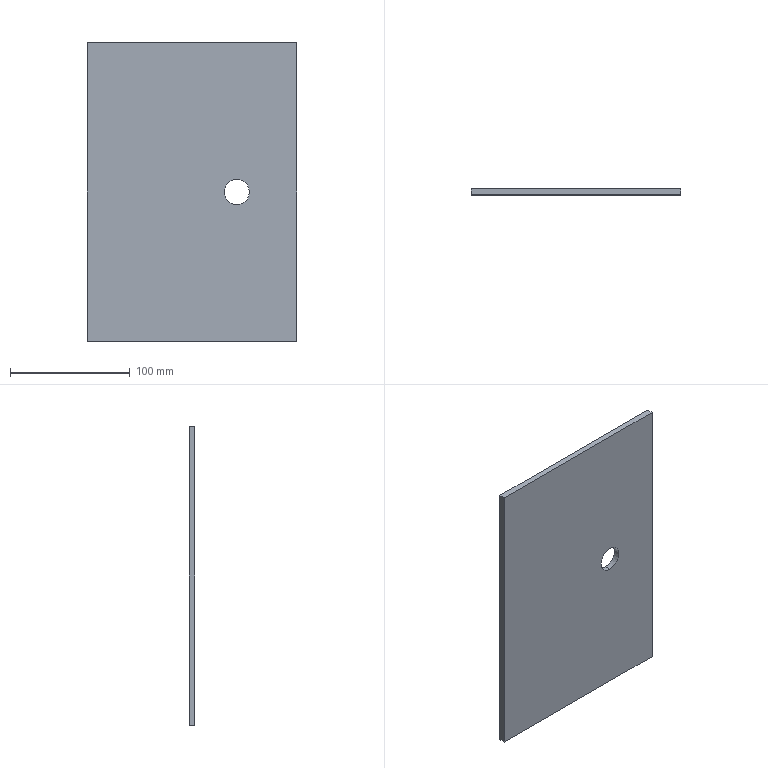Part | STEP file | Guide wheel mechanism revised.sldasm-Part-357 | 1 solid | 11 faces | box 175 x 5 x 250 mm | volume 216933 mm3 | plane 7 | cylinder 4 | commonest cylinder face diameters 6 x2 21 x2
STEP:
#1=CARTESIAN_POINT('',(0.,2.,54.));
#2=VERTEX_POINT('',#1);
#3=CARTESIAN_POINT('',(0.,2.,60.));
#4=VERTEX_POINT('',#3);
#5=CARTESIAN_POINT('',(0.,2.,57.));
#6=DIRECTION('',(0.,1.,0.));
#7=DIRECTION('',(0.,0.,1.));
#8=AXIS2_PLACEMENT_3D('',#5,#6,#7);
#9=CIRCLE('',#8,3.);
#10=EDGE_CURVE('',#2,#4,#9,.T.);
#11=ORIENTED_EDGE('',*,*,#10,.F.);
#12=CARTESIAN_POINT('',(0.,5.,54.));
#13=VERTEX_POINT('',#12);
#14=CARTESIAN_POINT('',(0.,2.,54.));
#15=DIRECTION('',(0.,1.,0.));
#16=VECTOR('',#15,1000.);
#17=LINE('',#14,#16);
#18=EDGE_CURVE('',#2,#13,#17,.T.);
#19=ORIENTED_EDGE('',*,*,#18,.T.);
#20=CARTESIAN_POINT('',(0.,5.,60.));
#21=VERTEX_POINT('',#20);
#22=CARTESIAN_POINT('',(0.,5.,57.));
#23=DIRECTION('',(0.,1.,0.));
#24=DIRECTION('',(0.,0.,1.));
#25=AXIS2_PLACEMENT_3D('',#22,#23,#24);
#26=CIRCLE('',#25,3.);
#27=EDGE_CURVE('',#13,#21,#26,.T.);
#28=ORIENTED_EDGE('',*,*,#27,.T.);
#29=CARTESIAN_POINT('',(0.,2.,60.));
#30=DIRECTION('',(0.,1.,0.));
#31=VECTOR('',#30,1000.);
#32=LINE('',#29,#31);
#33=EDGE_CURVE('',#4,#21,#32,.T.);
#34=ORIENTED_EDGE('',*,*,#33,.F.);
#35=EDGE_LOOP('',(#11,#19,#28,#34));
#36=FACE_OUTER_BOUND('',#35,.T.);
#37=CARTESIAN_POINT('',(0.,2.,57.));
#38=DIRECTION('',(0.,1.,0.));
#39=DIRECTION('',(0.,0.,1.));
#40=AXIS2_PLACEMENT_3D('',#37,#38,#39);
#41=CYLINDRICAL_SURFACE('',#40,3.);
#42=ADVANCED_FACE('',(#36),#41,.F.);
#43=CARTESIAN_POINT('',(0.,5.,-10.5));
#44=VERTEX_POINT('',#43);
#45=CARTESIAN_POINT('',(0.,5.,10.5));
#46=VERTEX_POINT('',#45);
#47=CARTESIAN_POINT('',(0.,5.,0.));
#48=DIRECTION('',(0.,1.,0.));
#49=DIRECTION('',(0.,0.,1.));
#50=AXIS2_PLACEMENT_3D('',#47,#48,#49);
#51=CIRCLE('',#50,10.5);
#52=EDGE_CURVE('',#44,#46,#51,.T.);
#53=ORIENTED_EDGE('',*,*,#52,.T.);
#54=CARTESIAN_POINT('',(0.,0.,10.5));
#55=VERTEX_POINT('',#54);
#56=CARTESIAN_POINT('',(0.,5.,10.5));
#57=DIRECTION('',(0.,-1.,0.));
#58=VECTOR('',#57,1000.);
#59=LINE('',#56,#58);
#60=EDGE_CURVE('',#46,#55,#59,.T.);
#61=ORIENTED_EDGE('',*,*,#60,.T.);
#62=CARTESIAN_POINT('',(0.,0.,-10.5));
#63=VERTEX_POINT('',#62);
#64=CARTESIAN_POINT('',(0.,0.,0.));
#65=DIRECTION('',(0.,1.,0.));
#66=DIRECTION('',(0.,0.,1.));
#67=AXIS2_PLACEMENT_3D('',#64,#65,#66);
#68=CIRCLE('',#67,10.5);
#69=EDGE_CURVE('',#63,#55,#68,.T.);
#70=ORIENTED_EDGE('',*,*,#69,.F.);
#71=CARTESIAN_POINT('',(0.,5.,-10.5));
#72=DIRECTION('',(0.,-1.,0.));
#73=VECTOR('',#72,1000.);
#74=LINE('',#71,#73);
#75=EDGE_CURVE('',#44,#63,#74,.T.);
#76=ORIENTED_EDGE('',*,*,#75,.F.);
#77=EDGE_LOOP('',(#53,#61,#70,#76));
#78=FACE_OUTER_BOUND('',#77,.T.);
#79=CARTESIAN_POINT('',(0.,5.,0.));
#80=DIRECTION('',(0.,-1.,0.));
#81=DIRECTION('',(0.,0.,-1.));
#82=AXIS2_PLACEMENT_3D('',#79,#80,#81);
#83=CYLINDRICAL_SURFACE('',#82,10.5);
#84=ADVANCED_FACE('',(#78),#83,.F.);
#85=CARTESIAN_POINT('',(50.,5.,-125.));
#86=VERTEX_POINT('',#85);
#87=CARTESIAN_POINT('',(50.,5.,125.));
#88=VERTEX_POINT('',#87);
#89=CARTESIAN_POINT('',(50.,5.,-125.));
#90=DIRECTION('',(0.,0.,1.));
#91=VECTOR('',#90,1000.);
#92=LINE('',#89,#91);
#93=EDGE_CURVE('',#86,#88,#92,.T.);
#94=ORIENTED_EDGE('',*,*,#93,.F.);
#95=CARTESIAN_POINT('',(-125.,5.,-125.));
#96=VERTEX_POINT('',#95);
#97=CARTESIAN_POINT('',(125.,5.,-125.));
#98=DIRECTION('',(-1.,0.,0.));
#99=VECTOR('',#98,1000.);
#100=LINE('',#97,#99);
#101=EDGE_CURVE('',#86,#96,#100,.T.);
#102=ORIENTED_EDGE('',*,*,#101,.T.);
#103=CARTESIAN_POINT('',(-125.,5.,125.));
#104=VERTEX_POINT('',#103);
#105=CARTESIAN_POINT('',(-125.,5.,125.));
#106=DIRECTION('',(0.,0.,1.));
#107=VECTOR('',#106,1000.);
#108=LINE('',#105,#107);
#109=EDGE_CURVE('',#96,#104,#108,.T.);
#110=ORIENTED_EDGE('',*,*,#109,.T.);
#111=CARTESIAN_POINT('',(125.,5.,125.));
#112=DIRECTION('',(1.,0.,0.));
#113=VECTOR('',#112,1000.);
#114=LINE('',#111,#113);
#115=EDGE_CURVE('',#104,#88,#114,.T.);
#116=ORIENTED_EDGE('',*,*,#115,.T.);
#117=EDGE_LOOP('',(#94,#102,#110,#116));
#118=FACE_OUTER_BOUND('',#117,.T.);
#119=CARTESIAN_POINT('',(0.,5.,57.));
#120=DIRECTION('',(0.,1.,0.));
#121=DIRECTION('',(0.,0.,1.));
#122=AXIS2_PLACEMENT_3D('',#119,#120,#121);
#123=CIRCLE('',#122,3.);
#124=EDGE_CURVE('',#21,#13,#123,.T.);
#125=ORIENTED_EDGE('',*,*,#124,.F.);
#126=ORIENTED_EDGE('',*,*,#27,.F.);
#127=EDGE_LOOP('',(#125,#126));
#128=FACE_BOUND('',#127,.T.);
#129=ORIENTED_EDGE('',*,*,#52,.F.);
#130=CARTESIAN_POINT('',(0.,5.,0.));
#131=DIRECTION('',(0.,1.,0.));
#132=DIRECTION('',(0.,0.,1.));
#133=AXIS2_PLACEMENT_3D('',#130,#131,#132);
#134=CIRCLE('',#133,10.5);
#135=EDGE_CURVE('',#46,#44,#134,.T.);
#136=ORIENTED_EDGE('',*,*,#135,.F.);
#137=EDGE_LOOP('',(#129,#136));
#138=FACE_BOUND('',#137,.T.);
#139=CARTESIAN_POINT('',(0.,5.,0.));
#140=DIRECTION('',(0.,1.,0.));
#141=DIRECTION('',(0.,0.,1.));
#142=AXIS2_PLACEMENT_3D('',#139,#140,#141);
#143=PLANE('',#142);
#144=ADVANCED_FACE('',(#118,#128,#138),#143,.T.);
#145=CARTESIAN_POINT('',(50.,0.,-125.));
#146=VERTEX_POINT('',#145);
#147=CARTESIAN_POINT('',(-125.,0.,-125.));
#148=VERTEX_POINT('',#147);
#149=CARTESIAN_POINT('',(125.,0.,-125.));
#150=DIRECTION('',(-1.,0.,0.));
#151=VECTOR('',#150,1000.);
#152=LINE('',#149,#151);
#153=EDGE_CURVE('',#146,#148,#152,.T.);
#154=ORIENTED_EDGE('',*,*,#153,.F.);
#155=CARTESIAN_POINT('',(50.,0.,125.));
#156=VERTEX_POINT('',#155);
#157=CARTESIAN_POINT('',(50.,0.,-125.));
#158=DIRECTION('',(0.,0.,-1.));
#159=VECTOR('',#158,1000.);
#160=LINE('',#157,#159);
#161=EDGE_CURVE('',#156,#146,#160,.T.);
#162=ORIENTED_EDGE('',*,*,#161,.F.);
#163=CARTESIAN_POINT('',(-125.,0.,125.));
#164=VERTEX_POINT('',#163);
#165=CARTESIAN_POINT('',(125.,0.,125.));
#166=DIRECTION('',(1.,0.,0.));
#167=VECTOR('',#166,1000.);
#168=LINE('',#165,#167);
#169=EDGE_CURVE('',#164,#156,#168,.T.);
#170=ORIENTED_EDGE('',*,*,#169,.F.);
#171=CARTESIAN_POINT('',(-125.,0.,125.));
#172=DIRECTION('',(0.,0.,1.));
#173=VECTOR('',#172,1000.);
#174=LINE('',#171,#173);
#175=EDGE_CURVE('',#148,#164,#174,.T.);
#176=ORIENTED_EDGE('',*,*,#175,.F.);
#177=EDGE_LOOP('',(#154,#162,#170,#176));
#178=FACE_OUTER_BOUND('',#177,.T.);
#179=ORIENTED_EDGE('',*,*,#69,.T.);
#180=CARTESIAN_POINT('',(0.,0.,0.));
#181=DIRECTION('',(0.,1.,0.));
#182=DIRECTION('',(0.,0.,1.));
#183=AXIS2_PLACEMENT_3D('',#180,#181,#182);
#184=CIRCLE('',#183,10.5);
#185=EDGE_CURVE('',#55,#63,#184,.T.);
#186=ORIENTED_EDGE('',*,*,#185,.T.);
#187=EDGE_LOOP('',(#179,#186));
#188=FACE_BOUND('',#187,.T.);
#189=CARTESIAN_POINT('',(0.,0.,0.));
#190=DIRECTION('',(0.,1.,0.));
#191=DIRECTION('',(0.,0.,1.));
#192=AXIS2_PLACEMENT_3D('',#189,#190,#191);
#193=PLANE('',#192);
#194=ADVANCED_FACE('',(#178,#188),#193,.F.);
#195=ORIENTED_EDGE('',*,*,#175,.T.);
#196=CARTESIAN_POINT('',(-125.,5.,125.));
#197=DIRECTION('',(0.,-1.,0.));
#198=VECTOR('',#197,1000.);
#199=LINE('',#196,#198);
#200=EDGE_CURVE('',#104,#164,#199,.T.);
#201=ORIENTED_EDGE('',*,*,#200,.F.);
#202=ORIENTED_EDGE('',*,*,#109,.F.);
#203=CARTESIAN_POINT('',(-125.,5.,-125.));
#204=DIRECTION('',(0.,-1.,0.));
#205=VECTOR('',#204,1000.);
#206=LINE('',#203,#205);
#207=EDGE_CURVE('',#96,#148,#206,.T.);
#208=ORIENTED_EDGE('',*,*,#207,.T.);
#209=EDGE_LOOP('',(#195,#201,#202,#208));
#210=FACE_OUTER_BOUND('',#209,.T.);
#211=CARTESIAN_POINT('',(-125.,5.,125.));
#212=DIRECTION('',(1.,0.,0.));
#213=DIRECTION('',(0.,0.,-1.));
#214=AXIS2_PLACEMENT_3D('',#211,#212,#213);
#215=PLANE('',#214);
#216=ADVANCED_FACE('',(#210),#215,.F.);
#217=ORIENTED_EDGE('',*,*,#169,.T.);
#218=CARTESIAN_POINT('',(50.,-0.001,125.));
#219=DIRECTION('',(0.,1.,0.));
#220=VECTOR('',#219,1000.);
#221=LINE('',#218,#220);
#222=EDGE_CURVE('',#156,#88,#221,.T.);
#223=ORIENTED_EDGE('',*,*,#222,.T.);
#224=ORIENTED_EDGE('',*,*,#115,.F.);
#225=ORIENTED_EDGE('',*,*,#200,.T.);
#226=EDGE_LOOP('',(#217,#223,#224,#225));
#227=FACE_OUTER_BOUND('',#226,.T.);
#228=CARTESIAN_POINT('',(125.,5.,125.));
#229=DIRECTION('',(0.,0.,-1.));
#230=DIRECTION('',(-1.,0.,0.));
#231=AXIS2_PLACEMENT_3D('',#228,#229,#230);
#232=PLANE('',#231);
#233=ADVANCED_FACE('',(#227),#232,.F.);
#234=ORIENTED_EDGE('',*,*,#101,.F.);
#235=CARTESIAN_POINT('',(50.,-0.001,-125.));
#236=DIRECTION('',(0.,1.,0.));
#237=VECTOR('',#236,1000.);
#238=LINE('',#235,#237);
#239=EDGE_CURVE('',#146,#86,#238,.T.);
#240=ORIENTED_EDGE('',*,*,#239,.F.);
#241=ORIENTED_EDGE('',*,*,#153,.T.);
#242=ORIENTED_EDGE('',*,*,#207,.F.);
#243=EDGE_LOOP('',(#234,#240,#241,#242));
#244=FACE_OUTER_BOUND('',#243,.T.);
#245=CARTESIAN_POINT('',(125.,5.,-125.));
#246=DIRECTION('',(0.,0.,1.));
#247=DIRECTION('',(1.,0.,0.));
#248=AXIS2_PLACEMENT_3D('',#245,#246,#247);
#249=PLANE('',#248);
#250=ADVANCED_FACE('',(#244),#249,.F.);
#251=ORIENTED_EDGE('',*,*,#60,.F.);
#252=ORIENTED_EDGE('',*,*,#135,.T.);
#253=ORIENTED_EDGE('',*,*,#75,.T.);
#254=ORIENTED_EDGE('',*,*,#185,.F.);
#255=EDGE_LOOP('',(#251,#252,#253,#254));
#256=FACE_OUTER_BOUND('',#255,.T.);
#257=CARTESIAN_POINT('',(0.,5.,0.));
#258=DIRECTION('',(0.,-1.,0.));
#259=DIRECTION('',(0.,0.,-1.));
#260=AXIS2_PLACEMENT_3D('',#257,#258,#259);
#261=CYLINDRICAL_SURFACE('',#260,10.5);
#262=ADVANCED_FACE('',(#256),#261,.F.);
#263=ORIENTED_EDGE('',*,*,#18,.F.);
#264=CARTESIAN_POINT('',(0.,2.,57.));
#265=DIRECTION('',(0.,1.,0.));
#266=DIRECTION('',(0.,0.,1.));
#267=AXIS2_PLACEMENT_3D('',#264,#265,#266);
#268=CIRCLE('',#267,3.);
#269=EDGE_CURVE('',#4,#2,#268,.T.);
#270=ORIENTED_EDGE('',*,*,#269,.F.);
#271=ORIENTED_EDGE('',*,*,#33,.T.);
#272=ORIENTED_EDGE('',*,*,#124,.T.);
#273=EDGE_LOOP('',(#263,#270,#271,#272));
#274=FACE_OUTER_BOUND('',#273,.T.);
#275=CARTESIAN_POINT('',(0.,2.,57.));
#276=DIRECTION('',(0.,1.,0.));
#277=DIRECTION('',(0.,0.,1.));
#278=AXIS2_PLACEMENT_3D('',#275,#276,#277);
#279=CYLINDRICAL_SURFACE('',#278,3.);
#280=ADVANCED_FACE('',(#274),#279,.F.);
#281=ORIENTED_EDGE('',*,*,#269,.T.);
#282=ORIENTED_EDGE('',*,*,#10,.T.);
#283=EDGE_LOOP('',(#281,#282));
#284=FACE_OUTER_BOUND('',#283,.T.);
#285=CARTESIAN_POINT('',(0.,2.,57.));
#286=DIRECTION('',(0.,1.,0.));
#287=DIRECTION('',(0.,0.,1.));
#288=AXIS2_PLACEMENT_3D('',#285,#286,#287);
#289=PLANE('',#288);
#290=ADVANCED_FACE('',(#284),#289,.T.);
#291=ORIENTED_EDGE('',*,*,#161,.T.);
#292=ORIENTED_EDGE('',*,*,#239,.T.);
#293=ORIENTED_EDGE('',*,*,#93,.T.);
#294=ORIENTED_EDGE('',*,*,#222,.F.);
#295=EDGE_LOOP('',(#291,#292,#293,#294));
#296=FACE_OUTER_BOUND('',#295,.T.);
#297=CARTESIAN_POINT('',(50.,-0.001,-125.));
#298=DIRECTION('',(-1.,0.,0.));
#299=DIRECTION('',(0.,0.,1.));
#300=AXIS2_PLACEMENT_3D('',#297,#298,#299);
#301=PLANE('',#300);
#302=ADVANCED_FACE('',(#296),#301,.F.);
#303=CLOSED_SHELL('',(#42,#84,#144,#194,#216,#233,#250,#262,#280,#290,#302));
#304=MANIFOLD_SOLID_BREP('',#303);
#305=CARTESIAN_POINT('',(0.,0.,0.));
#306=DIRECTION('',(0.,0.,1.));
#307=DIRECTION('',(1.,0.,0.));
#308=AXIS2_PLACEMENT_3D('',#305,#306,#307);
#309=(LENGTH_UNIT()NAMED_UNIT(*)SI_UNIT(.MILLI.,.METRE.));
#310=UNCERTAINTY_MEASURE_WITH_UNIT(LENGTH_MEASURE(0.00001),#309,'','');
#311=(NAMED_UNIT(*)PLANE_ANGLE_UNIT()SI_UNIT($,.RADIAN.));
#312=(NAMED_UNIT(*)SI_UNIT($,.STERADIAN.)SOLID_ANGLE_UNIT());
#313=(GEOMETRIC_REPRESENTATION_CONTEXT(3)GLOBAL_UNCERTAINTY_ASSIGNED_CONTEXT((#310))GLOBAL_UNIT_ASSIGNED_CONTEXT((#309,#311,#312))REPRESENTATION_CONTEXT('',''));
#314=ADVANCED_BREP_SHAPE_REPRESENTATION('',(#304,#308),#313);